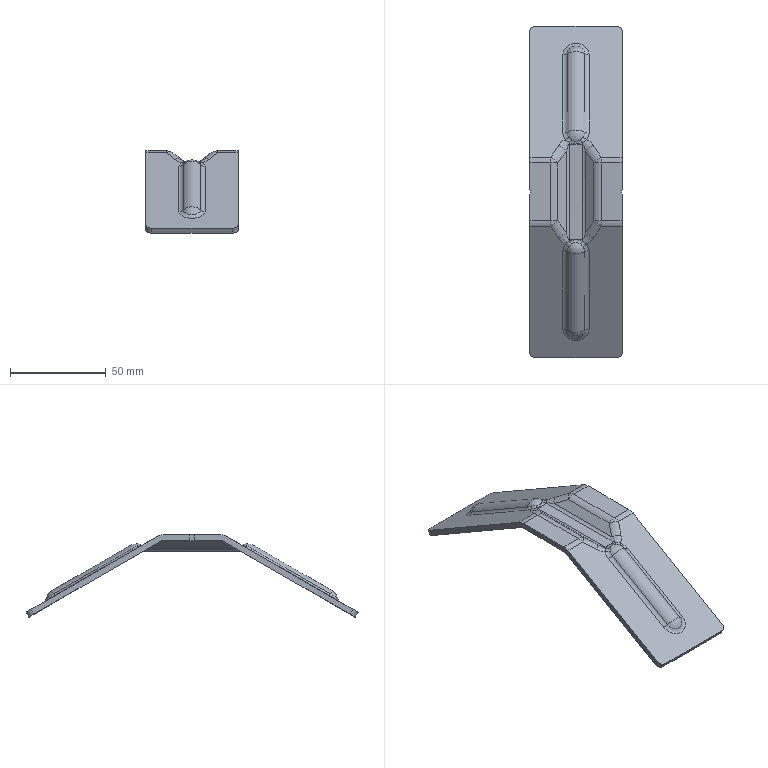Part | STEP file | 1_id90_x_t | 1 solid | 114 faces | box 48 x 173.045 x 42.934 mm | volume 28634 mm3 | cylinder 46 | spline 28 | plane 20 | torus 12 | sphere 8 | commonest cylinder face diameters 6 x14 12 x10 6.15 x6 12.15 x6 5.85 x2 6.3 x2